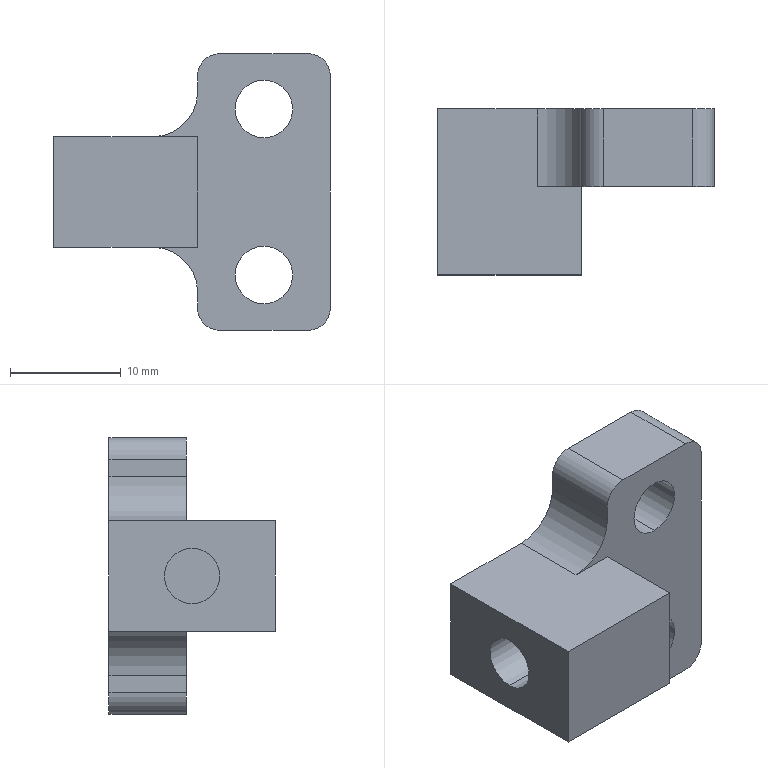NC program | Mastercam | posted with a generic post
Lines 21 to 1231 of 16956:
N230 T8 M6
N240 G0 G90 G17 G54 X-15.969 Y-26.116 A0. S7000 M3
N250 G43 H8 Z50. M8
N260 Z-7.15
N270 G1 Z-7.65 F600.
N280 X-16.17 Y-26.175 Z-7.658 F3000.
N290 X-16.376 Y-26.213 Z-7.665
N300 X-16.584 Y-26.229 Z-7.672
N310 X-16.794 Y-26.224 Z-7.68
N320 X-17.001 Y-26.196 Z-7.687
N330 X-17.205 Y-26.147 Z-7.694
N340 X-17.402 Y-26.077 Z-7.701
N350 X-17.591 Y-25.987 Z-7.709
N360 X-17.769 Y-25.877 Z-7.716
N370 X-17.935 Y-25.75 Z-7.723
N380 X-18.087 Y-25.605 Z-7.731
N390 X-18.223 Y-25.446 Z-7.738
N400 X-18.341 Y-25.274 Z-7.745
N410 X-18.441 Y-25.089 Z-7.753
N420 X-18.521 Y-24.896 Z-7.76
N430 X-19.329 Y-22.609
N440 X-19.66 Y-21.671 Z-7.859
N450 X-19.898 Y-20.996 Z-7.93
N460 X-19.975 Y-20.811 Z-7.95
N470 X-20.073 Y-20.636 Z-7.97
N480 X-20.189 Y-20.472 Z-7.99
N490 X-20.323 Y-20.323 Z-8.01
N500 X-20.568 Y-19.934
N510 X-20.758 Y-19.534
N520 X-20.912 Y-19.155
N530 X-21.033 Y-18.806
N540 X-21.124 Y-18.484
N550 X-21.193 Y-18.19
N560 X-21.244 Y-17.92
N570 X-21.281 Y-17.671
N580 X-21.331 Y-17.233
N590 X-21.36 Y-16.837
N600 X-21.378 Y-16.472
N610 X-21.389 Y-16.129
N620 X-21.395 Y-15.801
N630 X-21.398 Y-15.483
N640 X-21.399 Y-15.172
N650 Y-14.866
N660 X-21.398 Y-14.563
N670 X-21.396 Y-14.262
N680 X-21.395 Y-13.962
N690 X-21.393 Y-13.663
N700 X-21.391 Y-13.364
N710 X-21.389 Y-13.065
N720 X-21.387 Y-12.767
N730 X-21.385 Y-12.468
N740 X-21.383 Y-12.169
N750 X-21.381 Y-11.871
N760 X-21.379 Y-11.572
N770 X-21.377 Y-11.274
N780 X-21.375 Y-10.975
N790 X-21.373 Y-10.676
N800 X-21.371 Y-10.377
N810 X-21.369 Y-10.079
N820 X-21.367 Y-9.78
N830 X-21.365 Y-9.481
N840 X-21.363 Y-9.181
N850 X-21.361 Y-8.882
N860 X-21.359 Y-8.583
N870 X-21.357 Y-8.284
N880 X-21.355 Y-7.985
N890 X-21.353 Y-7.685
N900 X-21.35 Y-7.386
N910 X-21.348 Y-7.086
N920 X-21.346 Y-6.787
N930 X-21.344 Y-6.487
N940 X-21.342 Y-6.188
N950 X-21.34 Y-5.888
N960 X-21.338 Y-5.588
N970 X-21.336 Y-5.289
N980 X-21.334 Y-4.989
N990 X-21.332 Y-4.689
N1000 X-21.33 Y-4.389
N1010 X-21.328 Y-4.089
N1020 X-21.326 Y-3.789
N1030 X-21.324 Y-3.489
N1040 X-21.322 Y-3.189
N1050 X-21.32 Y-2.889
N1060 X-21.318 Y-2.589
N1070 X-21.315 Y-2.289
N1080 X-21.313 Y-1.989
N1090 X-21.311 Y-1.688
N1100 X-21.309 Y-1.388
N1110 X-21.307 Y-1.088
N1120 X-21.305 Y-.788
N1130 X-21.303 Y-.487
N1140 X-21.301 Y-.187
N1150 X-21.299 Y.114
N1160 X-21.297 Y.414
N1170 X-21.295 Y.715
N1180 X-21.293 Y1.015
N1190 X-21.291 Y1.316
N1200 X-21.289 Y1.616
N1210 X-21.287 Y1.917
N1220 X-21.285 Y2.218
N1230 X-21.282 Y2.519
N1240 X-21.28 Y2.819
N1250 X-21.278 Y3.12
N1260 X-21.276 Y3.421
N1270 X-21.274 Y3.722
N1280 X-21.272 Y4.023
N1290 X-21.27 Y4.323
N1300 X-21.268 Y4.624
N1310 X-21.266 Y4.925
N1320 X-21.264 Y5.226
N1330 X-21.262 Y5.527
N1340 X-21.26 Y5.828
N1350 X-21.258 Y6.129
N1360 X-21.256 Y6.43
N1370 X-21.254 Y6.732
N1380 X-21.251 Y7.033
N1390 X-21.249 Y7.334
N1400 X-21.247 Y7.635
N1410 X-21.245 Y7.936
N1420 X-21.243 Y8.237
N1430 X-21.241 Y8.539
N1440 X-21.239 Y8.84
N1450 X-21.237 Y9.141
N1460 X-21.235 Y9.443
N1470 X-21.233 Y9.744
N1480 X-21.231 Y10.045
N1490 X-21.229 Y10.347
N1500 X-21.227 Y10.648
N1510 X-21.225 Y10.95
N1520 X-21.223 Y11.251
N1530 X-21.22 Y11.552
N1540 X-21.218 Y11.854
N1550 X-21.216 Y12.155
N1560 X-21.214 Y12.457
N1570 X-21.212 Y12.759
N1580 X-21.21 Y13.06
N1590 X-21.208 Y13.362
N1600 X-21.206 Y13.663
N1610 X-21.204 Y13.965
N1620 X-21.202 Y14.267
N1630 X-21.2 Y14.568
N1640 X-21.198 Y14.87
N1650 X-21.196 Y15.172
N1660 X-21.194 Y15.474
N1670 X-21.191 Y15.775
N1680 X-21.179 Y16.217
N1690 X-21.138 Y16.554
N1700 X-21.065 Y16.892
N1710 X-20.962 Y17.226
N1720 X-20.83 Y17.552
N1730 X-20.673 Y17.865
N1740 X-20.492 Y18.163
N1750 X-20.293 Y18.443
N1760 X-20.077 Y18.703
N1770 X-19.849 Y18.944
N1780 X-19.612 Y19.164
N1790 X-19.369 Y19.364
N1800 X-19.122 Y19.546
N1810 X-18.873 Y19.709
N1820 X-18.625 Y19.855
N1830 X-18.378 Y19.986
N1840 X-18.134 Y20.103
N1850 X-17.894 Y20.207
N1860 X-17.657 Y20.3
N1870 X-17.425 Y20.382
N1880 X-17.198 Y20.455
N1890 X-16.765 Y20.576
N1900 X-16.347 Y20.673
N1910 X-15.945 Y20.751
N1920 X-15.556 Y20.814
N1930 X-15.179 Y20.864
N1940 X-14.814 Y20.904
N1950 X-14.458 Y20.936
N1960 X-14.111 Y20.962
N1970 X-13.77 Y20.983
N1980 X-13.436 Y20.999
N1990 X-13.107 Y21.013
N2000 X-12.782 Y21.023
N2010 X-12.462 Y21.031
N2020 X-12.144 Y21.038
N2030 X-11.828 Y21.043
N2040 X-11.516 Y21.046
N2050 X-11.204 Y21.049
N2060 X-10.895 Y21.05
N2070 X-10.587 Y21.051
N2080 X-10.28
N2090 X-9.973
N2100 X-9.668 Y21.05
N2110 X-9.363 Y21.049
N2120 X-9.059 Y21.048
N2130 X-8.755 Y21.047
N2140 X-8.451 Y21.045
N2150 X-8.147 Y21.043
N2160 X-7.844 Y21.042
N2170 X-7.541 Y21.04
N2180 X-7.237 Y21.038
N2190 X-6.934 Y21.036
N2200 X-6.631 Y21.034
N2210 X-6.328 Y21.032
N2220 X-6.025 Y21.03
N2230 X-5.722 Y21.028
N2240 X-5.419 Y21.026
N2250 X-5.116 Y21.024
N2260 X-4.813 Y21.022
N2270 X-4.511 Y21.02
N2280 X-4.208 Y21.018
N2290 X-3.905 Y21.016
N2300 X-3.602 Y21.014
N2310 X-3.299 Y21.012
N2320 X-2.995 Y21.01
N2330 X-2.691 Y21.009
N2340 X-2.386 Y21.007
N2350 X-2.081 Y21.006
N2360 X-1.776 Y21.005
N2370 X-1.47
N2380 X-1.165 Y21.004
N2390 X-.859 Y21.003
N2400 X-.553
N2410 X-.247 Y21.002
N2420 X.059
N2430 X.365
N2440 X.671
N2450 X.978 Y21.001
N2460 X1.284
N2470 X1.591
N2480 X1.897
N2490 X2.204
N2500 X2.51
N2510 X2.817 Y21.
N2520 X3.123
N2530 X3.43
N2540 X3.737
N2550 X4.043
N2560 X4.35
N2570 X4.657
N2580 X4.963
N2590 X5.27
N2600 X5.577
N2610 X5.883
N2620 X6.19
N2630 X6.497
N2640 X6.804
N2650 X7.11
N2660 X7.417
N2670 X7.724
N2680 X8.03
N2690 X8.337
N2700 X8.644
N2710 X8.951
N2720 X9.257
N2730 X9.564
N2740 X9.871
N2750 X10.177
N2760 X10.484
N2770 X10.791
N2780 X11.098
N2790 X11.404
N2800 X11.711
N2810 X12.018
N2820 X12.325
N2830 X12.631
N2840 X12.938
N2850 X13.245
N2860 X13.551
N2870 X13.858
N2880 X14.165
N2890 X14.472
N2900 X14.778
N2910 X15.085
N2920 X15.392
N2930 X15.794 Y20.993
N2940 X16.066 Y20.965
N2950 X16.343 Y20.916
N2960 X16.622 Y20.845
N2970 X16.9 Y20.753
N2980 X17.174 Y20.64
N2990 X17.442 Y20.508
N3000 X17.702 Y20.359
N3010 X17.951 Y20.193
N3020 X18.189 Y20.013
N3030 X18.413 Y19.821
N3040 X18.625 Y19.619
N3050 X18.822 Y19.409
N3060 X19.006 Y19.192
N3070 X19.177 Y18.971
N3080 X19.334 Y18.746
N3090 X19.479 Y18.519
N3100 X19.612 Y18.292
N3110 X19.733 Y18.065
N3120 X19.845 Y17.838
N3130 X19.946 Y17.613
N3140 X20.039 Y17.39
N3150 X20.197 Y16.958
N3160 X20.329 Y16.537
N3170 X20.438 Y16.125
N3180 X20.529 Y15.725
N3190 X20.605 Y15.335
N3200 X20.668 Y14.955
N3210 X20.72 Y14.584
N3220 X20.764 Y14.221
N3230 X20.801 Y13.865
N3240 X20.832 Y13.516
N3250 X20.858 Y13.173
N3260 X20.879 Y12.835
N3270 X20.898 Y12.501
N3280 X20.913 Y12.171
N3290 X20.926 Y11.844
N3300 X20.937 Y11.52
N3310 X20.947 Y11.198
N3320 X20.955 Y10.879
N3330 X20.961 Y10.562
N3340 X20.967 Y10.246
N3350 X20.972 Y9.931
N3360 X20.976 Y9.617
N3370 X20.98 Y9.305
N3380 X20.983 Y8.993
N3390 X20.985 Y8.682
N3400 X20.987 Y8.372
N3410 X20.989 Y8.062
N3420 X20.991 Y7.753
N3430 X20.992 Y7.444
N3440 X20.993 Y7.135
N3450 X20.994 Y6.827
N3460 X20.995 Y6.519
N3470 X20.996 Y6.211
N3480 Y5.903
N3490 X20.997 Y5.596
N3500 Y5.288
N3510 X20.998 Y4.981
N3520 Y4.673
N3530 Y4.366
N3540 X20.999 Y4.059
N3550 Y3.752
N3560 Y3.445
N3570 Y3.138
N3580 Y2.831
N3590 Y2.524
N3600 Y2.217
N3610 X21. Y1.91
N3620 Y1.604
N3630 Y1.297
N3640 Y.99
N3650 Y.683
N3660 Y.376
N3670 Y.07
N3680 Y-.237
N3690 Y-.544
N3700 Y-.851
N3710 Y-1.157
N3720 Y-1.464
N3730 Y-1.771
N3740 Y-2.078
N3750 Y-2.384
N3760 Y-2.691
N3770 Y-2.998
N3780 Y-3.305
N3790 Y-3.611
N3800 Y-3.918
N3810 Y-4.225
N3820 Y-4.532
N3830 Y-4.838
N3840 Y-5.145
N3850 Y-5.452
N3860 Y-5.759
N3870 Y-6.065
N3880 Y-6.372
N3890 Y-6.679
N3900 Y-6.985
N3910 Y-7.292
N3920 Y-7.599
N3930 Y-7.906
N3940 Y-8.212
N3950 Y-8.519
N3960 Y-8.826
N3970 Y-9.133
N3980 Y-9.439
N3990 Y-9.746
N4000 Y-10.053
N4010 Y-10.359
N4020 Y-10.666
N4030 Y-10.973
N4040 Y-11.28
N4050 Y-11.586
N4060 Y-11.893
N4070 Y-12.2
N4080 Y-12.507
N4090 Y-12.813
N4100 Y-13.12
N4110 Y-13.427
N4120 Y-13.733
N4130 Y-14.04
N4140 Y-14.347
N4150 Y-14.654
N4160 Y-14.96
N4170 Y-15.267
N4180 Y-15.593
N4190 X20.988 Y-15.859
N4200 X20.955 Y-16.132
N4210 X20.901 Y-16.41
N4220 X20.825 Y-16.689
N4230 X20.728 Y-16.967
N4240 X20.61 Y-17.24
N4250 X20.474 Y-17.506
N4260 X20.32 Y-17.763
N4270 X20.15 Y-18.01
N4280 X19.967 Y-18.244
N4290 X19.773 Y-18.466
N4300 X19.569 Y-18.674
N4310 X19.357 Y-18.868
N4320 X19.139 Y-19.049
N4330 X18.917 Y-19.216
N4340 X18.691 Y-19.37
N4350 X18.464 Y-19.512
N4360 X18.237 Y-19.642
N4370 X18.01 Y-19.761
N4380 X17.783 Y-19.87
N4390 X17.558 Y-19.969
N4400 X17.336 Y-20.06
N4410 X16.906 Y-20.215
N4420 X16.485 Y-20.343
N4430 X16.075 Y-20.45
N4440 X15.676 Y-20.539
N4450 X15.287 Y-20.613
N4460 X14.908 Y-20.675
N4470 X14.538 Y-20.726
N4480 X14.176 Y-20.769
N4490 X13.822 Y-20.805
N4500 X13.473 Y-20.835
N4510 X13.131 Y-20.861
N4520 X12.793 Y-20.882
N4530 X12.46 Y-20.9
N4540 X12.13 Y-20.915
N4550 X11.804 Y-20.928
N4560 X11.48 Y-20.939
N4570 X11.159 Y-20.948
N4580 X10.84 Y-20.956
N4590 X10.522 Y-20.962
N4600 X10.207 Y-20.968
N4610 X9.892 Y-20.973
N4620 X9.579 Y-20.977
N4630 X9.266 Y-20.98
N4640 X8.955 Y-20.983
N4650 X8.644 Y-20.986
N4660 X8.334 Y-20.988
N4670 X8.024 Y-20.989
N4680 X7.715 Y-20.991
N4690 X7.406 Y-20.992
N4700 X7.097 Y-20.993
N4710 X6.789 Y-20.994
N4720 X6.481 Y-20.995
N4730 X6.173 Y-20.996
N4740 X5.865 Y-20.997
N4750 X5.557
N4760 X5.25
N4770 X4.943 Y-20.998
N4780 X4.635
N4790 X4.328
N4800 X4.021 Y-20.999
N4810 X3.714
N4820 X3.407
N4830 X3.1
N4840 X2.793
N4850 X2.486
N4860 X2.179
N4870 X1.872 Y-21.
N4880 X1.566
N4890 X1.259
N4900 X.952
N4910 X.645
N4920 X.338
N4930 X.032
N4940 X-.275
N4950 X-.582
N4960 X-.889
N4970 X-1.195
N4980 X-1.502
N4990 X-1.809
N5000 X-2.116
N5010 X-2.422
N5020 X-2.729
N5030 X-3.036
N5040 X-3.343
N5050 X-3.649
N5060 X-3.956
N5070 X-4.263
N5080 X-4.57
N5090 X-4.876
N5100 X-5.183
N5110 X-5.49
N5120 X-5.797
N5130 X-6.103
N5140 X-6.41
N5150 X-6.717
N5160 X-7.023
N5170 X-7.33
N5180 X-7.637
N5190 X-7.944
N5200 X-8.25
N5210 X-8.557
N5220 X-8.864
N5230 X-9.171
N5240 X-9.477
N5250 X-9.784
N5260 X-10.091
N5270 X-10.397
N5280 X-10.704
N5290 X-11.011
N5300 X-11.318
N5310 X-11.624
N5320 X-11.931
N5330 X-12.238
N5340 X-12.545
N5350 X-12.851
N5360 X-13.158
N5370 X-13.465
N5380 X-13.771
N5390 X-14.078
N5400 X-14.385
N5410 X-14.692
N5420 X-14.998
N5430 X-15.305
N5440 X-15.591 Y-20.99
N5450 X-15.879 Y-20.96
N5460 X-16.167 Y-20.908
N5470 X-16.453 Y-20.836
N5480 X-16.736 Y-20.744
N5490 X-17.013 Y-20.632
N5500 X-17.283 Y-20.501
N5510 X-17.543 Y-20.354
N5520 X-17.794 Y-20.191
N5530 X-18.033 Y-20.014
N5540 X-18.259 Y-19.825
N5550 X-18.473 Y-19.625
N5560 X-18.673 Y-19.418
N5570 X-18.86 Y-19.203
N5580 X-19.033 Y-18.983
N5590 X-19.194 Y-18.759
N5600 X-19.342 Y-18.533
N5610 X-19.477 Y-18.306
N5620 X-19.602 Y-18.078
N5630 X-19.716 Y-17.851
N5640 X-19.82 Y-17.624
N5650 X-19.915 Y-17.4
N5660 X-20.001 Y-17.178
N5670 X-20.149 Y-16.748
N5680 X-20.271 Y-16.329
N5690 X-20.373 Y-15.92
N5700 X-20.457 Y-15.522
N5710 X-20.526 Y-15.134
N5720 X-20.584 Y-14.756
N5730 X-20.631 Y-14.387
N5740 X-20.67 Y-14.026
N5750 X-20.703 Y-13.672
N5760 X-20.73 Y-13.324
N5770 X-20.752 Y-12.982
N5780 X-20.771 Y-12.645
N5790 X-20.786 Y-12.312
N5800 X-20.799 Y-11.982
N5810 X-20.809 Y-11.656
N5820 X-20.817 Y-11.333
N5830 X-20.824 Y-11.012
N5840 X-20.83 Y-10.693
N5850 X-20.834 Y-10.376
N5860 X-20.837 Y-10.06
N5870 X-20.84 Y-9.746
N5880 X-20.842 Y-9.433
N5890 X-20.843 Y-9.12
N5900 X-20.844 Y-8.809
N5910 Y-8.498
N5920 Y-8.188
N5930 Y-7.878
N5940 X-20.843 Y-7.569
N5950 X-20.842 Y-7.26
N5960 X-20.841 Y-6.952
N5970 X-20.84 Y-6.643
N5980 X-20.839 Y-6.335
N5990 X-20.837 Y-6.027
N6000 X-20.836 Y-5.72
N6010 X-20.834 Y-5.412
N6020 X-20.832 Y-5.105
N6030 X-20.831 Y-4.797
N6040 X-20.829 Y-4.49
N6050 X-20.827 Y-4.183
N6060 X-20.825 Y-3.876
N6070 X-20.823 Y-3.569
N6080 X-20.821 Y-3.262
N6090 X-20.819 Y-2.955
N6100 X-20.817 Y-2.648
N6110 X-20.815 Y-2.341
N6120 X-20.813 Y-2.034
N6130 X-20.811 Y-1.727
N6140 X-20.809 Y-1.421
N6150 X-20.807 Y-1.114
N6160 X-20.805 Y-.807
N6170 X-20.803 Y-.5
N6180 X-20.801 Y-.193
N6190 X-20.799 Y.113
N6200 X-20.797 Y.42
N6210 X-20.795 Y.727
N6220 X-20.793 Y1.034
N6230 X-20.79 Y1.34
N6240 X-20.788 Y1.647
N6250 X-20.786 Y1.954
N6260 X-20.784 Y2.261
N6270 X-20.782 Y2.567
N6280 X-20.78 Y2.874
N6290 X-20.778 Y3.181
N6300 X-20.776 Y3.488
N6310 X-20.774 Y3.794
N6320 X-20.772 Y4.101
N6330 X-20.769 Y4.408
N6340 X-20.767 Y4.715
N6350 X-20.765 Y5.021
N6360 X-20.763 Y5.328
N6370 X-20.761 Y5.635
N6380 X-20.759 Y5.941
N6390 X-20.757 Y6.248
N6400 X-20.755 Y6.555
N6410 X-20.753 Y6.862
N6420 X-20.751 Y7.168
N6430 X-20.748 Y7.475
N6440 X-20.746 Y7.782
N6450 X-20.744 Y8.089
N6460 X-20.742 Y8.395
N6470 X-20.74 Y8.702
N6480 X-20.738 Y9.009
N6490 X-20.736 Y9.315
N6500 X-20.734 Y9.622
N6510 X-20.732 Y9.929
N6520 X-20.729 Y10.236
N6530 X-20.727 Y10.542
N6540 X-20.725 Y10.849
N6550 X-20.723 Y11.156
N6560 X-20.721 Y11.462
N6570 X-20.719 Y11.769
N6580 X-20.717 Y12.076
N6590 X-20.715 Y12.383
N6600 X-20.713 Y12.689
N6610 X-20.711 Y12.996
N6620 X-20.708 Y13.303
N6630 X-20.706 Y13.61
N6640 X-20.704 Y13.92
N6650 X-20.701 Y14.136
N6660 X-20.687 Y14.412
N6670 X-20.658 Y14.697
N6680 X-20.614 Y14.984
N6690 X-20.554 Y15.271
N6700 X-20.479 Y15.553
N6710 X-20.388 Y15.832
N6720 X-20.282 Y16.105
N6730 X-20.162 Y16.37
N6740 X-20.028 Y16.628
N6750 X-19.882 Y16.878
N6760 X-19.724 Y17.117
N6770 X-19.556 Y17.346
N6780 X-19.379 Y17.565
N6790 X-19.193 Y17.773
N6800 X-19. Y17.971
N6810 X-18.802 Y18.157
N6820 X-18.598 Y18.333
N6830 X-18.391 Y18.498
N6840 X-18.179 Y18.652
N6850 X-17.966 Y18.797
N6860 X-17.751 Y18.932
N6870 X-17.536 Y19.057
N6880 X-17.319 Y19.174
N6890 X-17.103 Y19.282
N6900 X-16.887 Y19.383
N6910 X-16.467 Y19.558
N6920 X-16.051 Y19.709
N6930 X-15.642 Y19.838
N6940 X-15.241 Y19.947
N6950 X-14.847 Y20.04
N6960 X-14.461 Y20.119
N6970 X-14.082 Y20.186
N6980 X-13.711 Y20.243
N6990 X-13.347 Y20.291
N7000 X-12.989 Y20.331
N7010 X-12.636 Y20.365
N7020 X-12.29 Y20.394
N7030 X-11.948 Y20.418
N7040 X-11.61 Y20.438
N7050 X-11.276 Y20.455
N7060 X-10.946 Y20.469
N7070 X-10.619 Y20.481
N7080 X-10.295 Y20.49
N7090 X-9.972 Y20.498
N7100 X-9.653 Y20.505
N7110 X-9.334 Y20.51
N7120 X-9.018 Y20.514
N7130 X-8.703 Y20.517
N7140 X-8.389 Y20.52
N7150 X-8.075 Y20.522
N7160 X-7.763 Y20.523
N7170 X-7.452 Y20.524
N7180 X-7.141
N7190 X-6.831
N7200 X-6.522 Y20.523
N7210 X-6.212
N7220 X-5.903 Y20.522
N7230 X-5.595 Y20.521
N7240 X-5.287 Y20.52
N7250 X-4.979 Y20.519
N7260 X-4.672 Y20.517
N7270 X-4.365 Y20.516
N7280 X-4.059 Y20.515
N7290 X-3.753 Y20.513
N7300 X-3.447 Y20.512
N7310 X-3.141 Y20.511
N7320 X-2.835 Y20.51
N7330 X-2.529 Y20.509
N7340 X-2.223 Y20.508
N7350 X-1.917 Y20.507
N7360 X-1.611 Y20.506
N7370 X-1.305
N7380 X-.999 Y20.505
N7390 X-.693
N7400 X-.387 Y20.504
N7410 X-.081
N7420 X.226 Y20.503
N7430 X.532
N7440 X.838 Y20.502
N7450 X1.144
N7460 X1.451
N7470 X1.757
N7480 X2.064 Y20.501
N7490 X2.37
N7500 X2.677
N7510 X2.983
N7520 X3.29
N7530 X3.596
N7540 X3.903
N7550 X4.21
N7560 X4.516
N7570 X4.823 Y20.5
N7580 X5.13
N7590 X5.436
N7600 X5.743
N7610 X6.05
N7620 X6.356
N7630 X6.663
N7640 X6.97
N7650 X7.276
N7660 X7.583
N7670 X7.89
N7680 X8.196
N7690 X8.503
N7700 X8.81
N7710 X9.117
N7720 X9.423
N7730 X9.73
N7740 X10.037
N7750 X10.343
N7760 X10.65
N7770 X10.957
N7780 X11.264
N7790 X11.57
N7800 X11.877
N7810 X12.184
N7820 X12.49
N7830 X12.797
N7840 X13.104
N7850 X13.411
N7860 X13.809 Y20.496
N7870 X14.085 Y20.481
N7880 X14.367 Y20.452
N7890 X14.651 Y20.409
N7900 X14.934 Y20.35
N7910 X15.214 Y20.277
N7920 X15.489 Y20.189
N7930 X15.759 Y20.088
N7940 X16.023 Y19.972
N7950 X16.28 Y19.844
N7960 X16.528 Y19.704
N7970 X16.767 Y19.553
N7980 X16.997 Y19.393
N7990 X17.218 Y19.223
N8000 X17.428 Y19.045
N8010 X17.628 Y18.86
N8020 X17.818 Y18.669
N8030 X17.998 Y18.473
N8040 X18.168 Y18.272
N8050 X18.329 Y18.068
N8060 X18.479 Y17.861
N8070 X18.621 Y17.652
N8080 X18.753 Y17.442
N8090 X18.877 Y17.231
N8100 X18.993 Y17.019
N8110 X19.1 Y16.807
N8120 X19.291 Y16.393
N8130 X19.457 Y15.982
N8140 X19.601 Y15.576
N8150 X19.725 Y15.176
N8160 X19.832 Y14.782
N8170 X19.924 Y14.395
N8180 X20.003 Y14.015
N8190 X20.071 Y13.642
N8200 X20.13 Y13.275
N8210 X20.18 Y12.915
N8220 X20.224 Y12.56
N8230 X20.261 Y12.21
N8240 X20.294 Y11.865
N8250 X20.322 Y11.524
N8260 X20.346 Y11.188
N8270 X20.367 Y10.854
N8280 X20.385 Y10.524
N8290 X20.4 Y10.197
N8300 X20.413 Y9.872
N8310 X20.425 Y9.55
N8320 X20.435 Y9.229
N8330 X20.444 Y8.91
N8340 X20.451 Y8.593
N8350 X20.458 Y8.277
N8360 X20.464 Y7.962
N8370 X20.468 Y7.648
N8380 X20.473 Y7.335
N8390 X20.476 Y7.023
N8400 X20.48 Y6.712
N8410 X20.482 Y6.401
N8420 X20.485 Y6.091
N8430 X20.487 Y5.781
N8440 X20.489 Y5.472
N8450 X20.49 Y5.163
N8460 X20.491 Y4.854
N8470 X20.493 Y4.545
N8480 X20.494 Y4.237
N8490 Y3.929
N8500 X20.495 Y3.621
N8510 X20.496 Y3.313
N8520 Y3.006
N8530 X20.497 Y2.698
N8540 Y2.391
N8550 X20.498 Y2.084
N8560 Y1.776
N8570 Y1.469
N8580 X20.499 Y1.162
N8590 Y.855
N8600 Y.548
N8610 Y.241
N8620 Y-.066
N8630 Y-.373
N8640 Y-.679
N8650 Y-.986
N8660 X20.5 Y-1.293
N8670 Y-1.6
N8680 Y-1.907
N8690 Y-2.214
N8700 Y-2.52
N8710 Y-2.827
N8720 Y-3.134
N8730 Y-3.441
N8740 Y-3.748
N8750 Y-4.054
N8760 Y-4.361
N8770 Y-4.668
N8780 Y-4.975
N8790 Y-5.281
N8800 Y-5.588
N8810 Y-5.895
N8820 Y-6.202
N8830 Y-6.508
N8840 Y-6.815
N8850 Y-7.122
N8860 Y-7.429
N8870 Y-7.735
N8880 Y-8.042
N8890 Y-8.349
N8900 Y-8.655
N8910 Y-8.962
N8920 Y-9.269
N8930 Y-9.576
N8940 Y-9.882
N8950 Y-10.189
N8960 Y-10.496
N8970 Y-10.803
N8980 Y-11.109
N8990 Y-11.416
N9000 Y-11.723
N9010 Y-12.029
N9020 Y-12.336
N9030 Y-12.643
N9040 Y-12.95
N9050 Y-13.256
N9060 Y-13.563
N9070 X20.496 Y-13.815
N9080 X20.481 Y-14.091
N9090 X20.451 Y-14.373
N9100 X20.408 Y-14.657
N9110 X20.349 Y-14.939
N9120 X20.275 Y-15.219
N9130 X20.187 Y-15.495
N9140 X20.085 Y-15.765
N9150 X19.97 Y-16.028
N9160 X19.841 Y-16.285
N9170 X19.701 Y-16.533
N9180 X19.55 Y-16.772
N9190 X19.389 Y-17.001
N9200 X19.219 Y-17.222
N9210 X19.042 Y-17.432
N9220 X18.856 Y-17.632
N9230 X18.665 Y-17.822
N9240 X18.468 Y-18.002
N9250 X18.268 Y-18.172
N9260 X18.064 Y-18.332
N9270 X17.857 Y-18.482
N9280 X17.648 Y-18.624
N9290 X17.438 Y-18.756
N9300 X17.226 Y-18.879
N9310 X17.015 Y-18.995
N9320 X16.803 Y-19.103
N9330 X16.389 Y-19.293
N9340 X15.978 Y-19.459
N9350 X15.572 Y-19.602
N9360 X15.172 Y-19.726
N9370 X14.778 Y-19.833
N9380 X14.391 Y-19.924
N9390 X14.011 Y-20.004
N9400 X13.638 Y-20.072
N9410 X13.272 Y-20.13
N9420 X12.911 Y-20.181
N9430 X12.556 Y-20.224
N9440 X12.206 Y-20.262
N9450 X11.861 Y-20.294
N9460 X11.521 Y-20.322
N9470 X11.184 Y-20.346
N9480 X10.851 Y-20.367
N9490 X10.521 Y-20.385
N9500 X10.194 Y-20.4
N9510 X9.869 Y-20.414
N9520 X9.546 Y-20.425
N9530 X9.226 Y-20.435
N9540 X8.907 Y-20.444
N9550 X8.59 Y-20.451
N9560 X8.274 Y-20.458
N9570 X7.959 Y-20.464
N9580 X7.645 Y-20.468
N9590 X7.332 Y-20.473
N9600 X7.02 Y-20.476
N9610 X6.709 Y-20.48
N9620 X6.398 Y-20.482
N9630 X6.088 Y-20.485
N9640 X5.778 Y-20.487
N9650 X5.468 Y-20.489
N9660 X5.159 Y-20.49
N9670 X4.851 Y-20.491
N9680 X4.542 Y-20.493
N9690 X4.234 Y-20.494
N9700 X3.926
N9710 X3.618 Y-20.495
N9720 X3.31 Y-20.496
N9730 X3.003
N9740 X2.695 Y-20.497
N9750 X2.388
N9760 X2.08 Y-20.498
N9770 X1.773
N9780 X1.466
N9790 X1.159 Y-20.499
N9800 X.852
N9810 X.545
N9820 X.238
N9830 X-.069
N9840 X-.376
N9850 X-.683
N9860 X-.99
N9870 X-1.296 Y-20.5
N9880 X-1.603
N9890 X-1.91
N9900 X-2.217
N9910 X-2.524
N9920 X-2.83
N9930 X-3.137
N9940 X-3.444
N9950 X-3.751
N9960 X-4.057
N9970 X-4.364
N9980 X-4.671
N9990 X-4.978
N100 X-5.284
N110 X-5.591
N120 X-5.898
N130 X-6.205
N140 X-6.511
N150 X-6.818
N160 X-7.125
N170 X-7.432
N180 X-7.738
N190 X-8.045
N200 X-8.352
N210 X-8.659
N220 X-8.965
N230 X-9.272
N240 X-9.579
N250 X-9.886
N260 X-10.192
N270 X-10.499
N280 X-10.806
N290 X-11.112
N300 X-11.419
N310 X-11.726
N320 X-12.033
N330 X-12.339
N340 X-12.646
N350 X-12.953
N360 X-13.26
N370 X-13.671 Y-20.495
N380 X-13.942 Y-20.48
N390 X-14.22 Y-20.451
N400 X-14.501 Y-20.409
N410 X-14.782 Y-20.352
N420 X-15.061 Y-20.28
N430 X-15.336 Y-20.194
N440 X-15.605 Y-20.095
N450 X-15.869 Y-19.982
N460 X-16.126 Y-19.856
N470 X-16.376 Y-19.717
N480 X-16.616 Y-19.569
N490 X-16.847 Y-19.409
N500 X-17.068 Y-19.242
N510 X-17.281 Y-19.065
N520 X-17.482 Y-18.882
N530 X-17.675 Y-18.691
N540 X-17.856 Y-18.496
N550 X-18.028 Y-18.296
N560 X-18.19 Y-18.093
N570 X-18.343 Y-17.886
N580 X-18.486 Y-17.677
N590 X-18.62 Y-17.466
N600 X-18.745 Y-17.255
N610 X-18.862 Y-17.043
N620 X-18.971 Y-16.831
N630 X-19.165 Y-16.415
N640 X-19.332 Y-16.003
N650 X-19.477 Y-15.595
N660 X-19.602 Y-15.193
N670 X-19.71 Y-14.797
N680 X-19.802 Y-14.408
N690 X-19.882 Y-14.027
N700 X-19.949 Y-13.652
N710 X-20.008 Y-13.283
N720 X-20.057 Y-12.921
N730 X-20.1 Y-12.564
N740 X-20.136 Y-12.213
N750 X-20.168 Y-11.867
N760 X-20.194 Y-11.525
N770 X-20.217 Y-11.188
N780 X-20.236 Y-10.853
N790 X-20.252 Y-10.523
N800 X-20.266 Y-10.195
N810 X-20.278 Y-9.869
N820 X-20.288 Y-9.546
N830 X-20.296 Y-9.225
N840 X-20.303 Y-8.906
N850 X-20.308 Y-8.588
N860 X-20.313 Y-8.272
N870 X-20.317 Y-7.956
N880 X-20.319 Y-7.642
N890 X-20.322 Y-7.329
N900 X-20.323 Y-7.017
N910 X-20.325 Y-6.705
N920 Y-6.394
N930 X-20.326 Y-6.084
N940 Y-5.774
N950 X-20.325 Y-5.465
N960 Y-5.155
N970 X-20.324 Y-4.847
N980 X-20.323 Y-4.538
N990 X-20.322 Y-4.23
N1000 X-20.321 Y-3.922
N1010 X-20.32 Y-3.614
N1020 X-20.318 Y-3.306
N1030 X-20.317 Y-2.998
N1040 X-20.315 Y-2.691
N1050 X-20.313 Y-2.383
N1060 X-20.312 Y-2.076
N1070 X-20.31 Y-1.769
N1080 X-20.308 Y-1.462
N1090 X-20.306 Y-1.155
N1100 X-20.304 Y-.848
N1110 X-20.302 Y-.541
N1120 X-20.3 Y-.234
N1130 X-20.298 Y.073
N1140 X-20.296 Y.38
N1150 X-20.294 Y.687
N1160 X-20.292 Y.994
N1170 X-20.29 Y1.301
N1180 X-20.288 Y1.608
N1190 X-20.286 Y1.914
N1200 X-20.284 Y2.221
N1210 X-20.282 Y2.528
N1220 X-20.28 Y2.835
N1230 X-20.278 Y3.142
N1240 X-20.276 Y3.448
N1250 X-20.274 Y3.755
N1260 X-20.272 Y4.062
N1270 X-20.27 Y4.369
N1280 X-20.268 Y4.675
N1290 X-20.265 Y4.982
N1300 X-20.263 Y5.289
N1310 X-20.261 Y5.596
N1320 X-20.259 Y5.902
N1330 X-20.257 Y6.209
N1340 X-20.255 Y6.516
N1350 X-20.253 Y6.823
N1360 X-20.251 Y7.129
N1370 X-20.249 Y7.436
N1380 X-20.247 Y7.743
N1390 X-20.244 Y8.049
N1400 X-20.242 Y8.356
N1410 X-20.24 Y8.663
N1420 X-20.238 Y8.97
N1430 X-20.236 Y9.276
N1440 X-20.234 Y9.583
N1450 X-20.232 Y9.89
N1460 X-20.23 Y10.197
N1470 X-20.228 Y10.503
N1480 X-20.226 Y10.81
N1490 X-20.223 Y11.117
N1500 X-20.221 Y11.423
N1510 X-20.219 Y11.73
N1520 X-20.217 Y12.038
N1530 X-20.213 Y12.377
N1540 X-20.199 Y12.793
N1550 X-20.183 Y13.03
N1560 X-20.159 Y13.279
N1570 X-20.125 Y13.535
N1580 X-20.08 Y13.796
N1590 X-20.023 Y14.059
N1600 X-19.956 Y14.322
N1610 X-19.876 Y14.584
N1620 X-19.784 Y14.843
N1630 X-19.682 Y15.097
N1640 X-19.568 Y15.347
N1650 X-19.443 Y15.592
N1660 X-19.309 Y15.83
N1670 X-19.164 Y16.062
N1680 X-19.012 Y16.284
N1690 X-18.85 Y16.5
N1700 X-18.683 Y16.706
N1710 X-18.507 Y16.905
N1720 X-18.327 Y17.094
N1730 X-18.14 Y17.276
N1740 X-17.95 Y17.449
N1750 X-17.755 Y17.612
N1760 X-17.557 Y17.768
N1770 X-17.357 Y17.915
N1780 X-17.154 Y18.055
N1790 X-16.95 Y18.185
N1800 X-16.744 Y18.309
N1810 X-16.539 Y18.425
N1820 X-16.133 Y18.634
N1830 X-15.727 Y18.817
N1840 X-15.324 Y18.978
N1850 X-14.924 Y19.12
N1860 X-14.528 Y19.243
N1870 X-14.138 Y19.35
N1880 X-13.754 Y19.443
N1890 X-13.376 Y19.524
N1900 X-13.003 Y19.594
N1910 X-12.636 Y19.655
N1920 X-12.275 Y19.707
N1930 X-11.918 Y19.753
N1940 X-11.567 Y19.792
N1950 X-11.22 Y19.826
N1960 X-10.878 Y19.855
N1970 X-10.539 Y19.88
N1980 X-10.203 Y19.901
N1990 X-9.871 Y19.919
N2000 X-9.542 Y19.935
N2010 X-9.215 Y19.948
N2020 X-8.891 Y19.96
N2030 X-8.569 Y19.969
N2040 X-8.248 Y19.977
N2050 X-7.929 Y19.984
N2060 X-7.612 Y19.99
N2070 X-7.296 Y19.994
N2080 X-6.981 Y19.998
N2090 X-6.667 Y20.001
N2100 X-6.354 Y20.003
N2110 X-6.043 Y20.005
N2120 X-5.732 Y20.006
N2130 X-5.421 Y20.007
N2140 X-5.111 Y20.008
N2150 X-4.802
N2160 X-4.494 Y20.009
N2170 X-4.185
N2180 X-3.877 Y20.008
N2190 X-3.57
N2200 X-3.262
N2210 X-2.955
N2220 X-2.648 Y20.007
N2230 X-2.341
N2240 X-2.035 Y20.006
N2250 X-1.728
N2260 X-1.421 Y20.005
N2270 X-1.115
N2280 X-.808
N2290 X-.501 Y20.004
N2300 X-.195
N2310 X.112
N2320 X.418 Y20.003
N2330 X.725
N2340 X1.031
N2350 X1.338 Y20.002
N2360 X1.644
N2370 X1.951
N2380 X2.257
N2390 X2.564
N2400 X2.87 Y20.001
N2410 X3.177
N2420 X3.483
N2430 X3.79